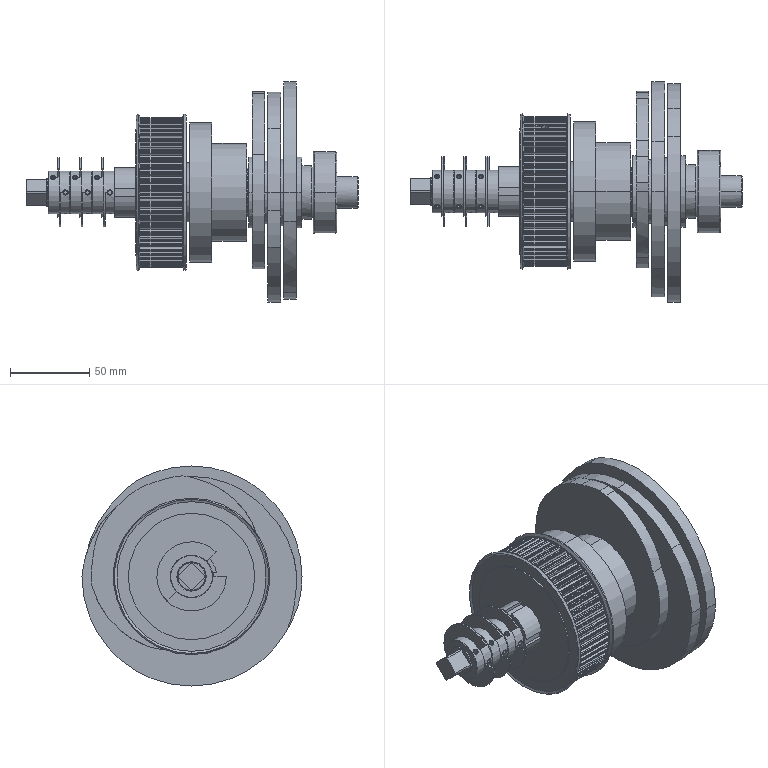Part | NX | 19 solids | 988 faces | box 210 x 139.21 x 139.21 mm | volume 759979 mm3 | cylinder 727 | plane 130 | cone 78 | spline 29 | torus 24 | commonest cylinder face diameters 0.5 x124 1.1 x124 6.55 x124 94.53 x88 90.99 x63 2.5 x24